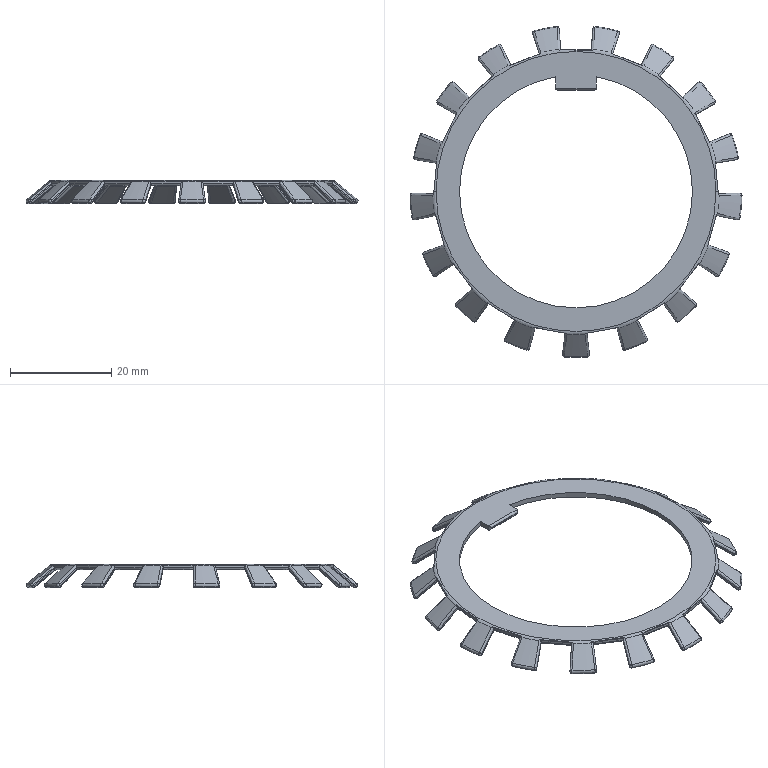Part | SolidWorks | features Fillet 3, ICE 2, CirPattern 1, Revolution 1 | 1 solid | 339 faces | box 65.578 x 65.38 x 4.578 mm | volume 1295 mm3 | spline 204 | plane 56 | torus 38 | cone 34 | cylinder 7 | commonest cylinder face diameters 0.8 x4 46 x3